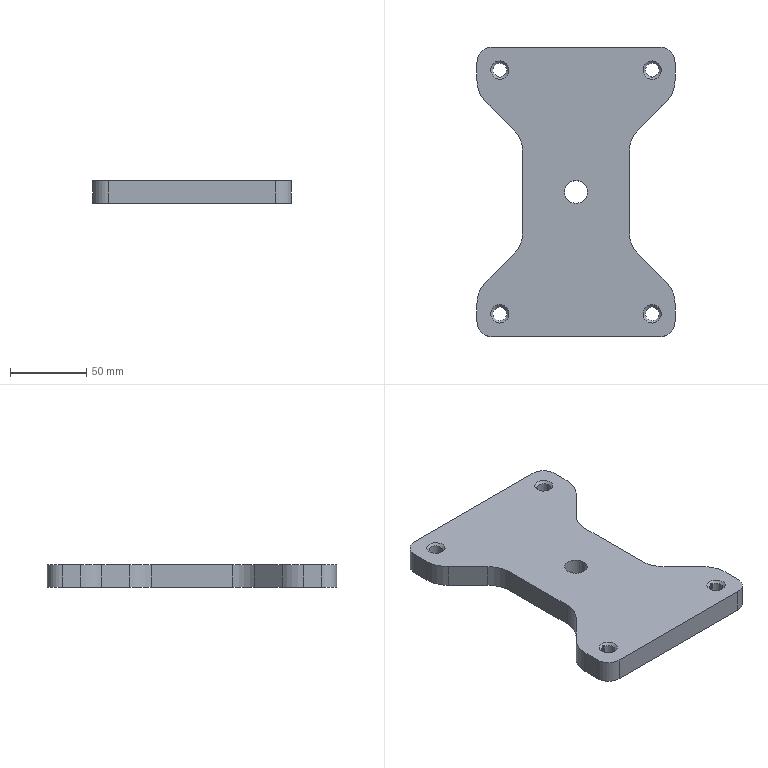Part | STEP file | YBQDJ-YY-8 | 1 solid | 47 faces | box 130 x 190 x 15 mm | volume 272574 mm3 | cylinder 29 | plane 14 | cone 4 | commonest cylinder face diameters 4 x8 40 x8 1 x4 9 x4 20 x4 15 x1